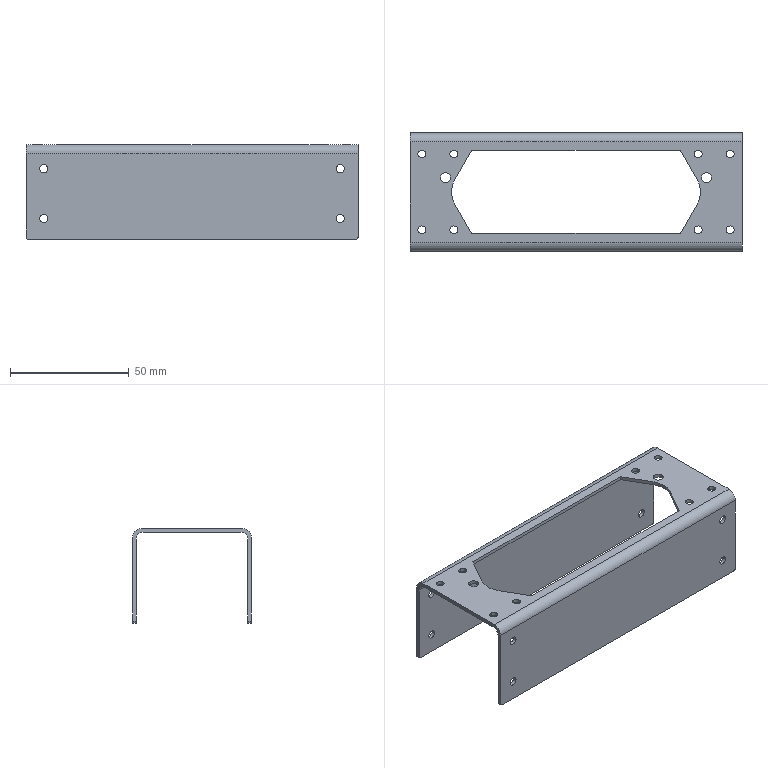Part | STEP file | Corpo | 1 solid | 62 faces | box 140 x 50 x 40 mm | volume 20970 mm3 | cylinder 46 | plane 16 | commonest cylinder face diameters 3.3 x16 3.5 x16 2 x4 4.2 x4 6 x2 7.5 x2